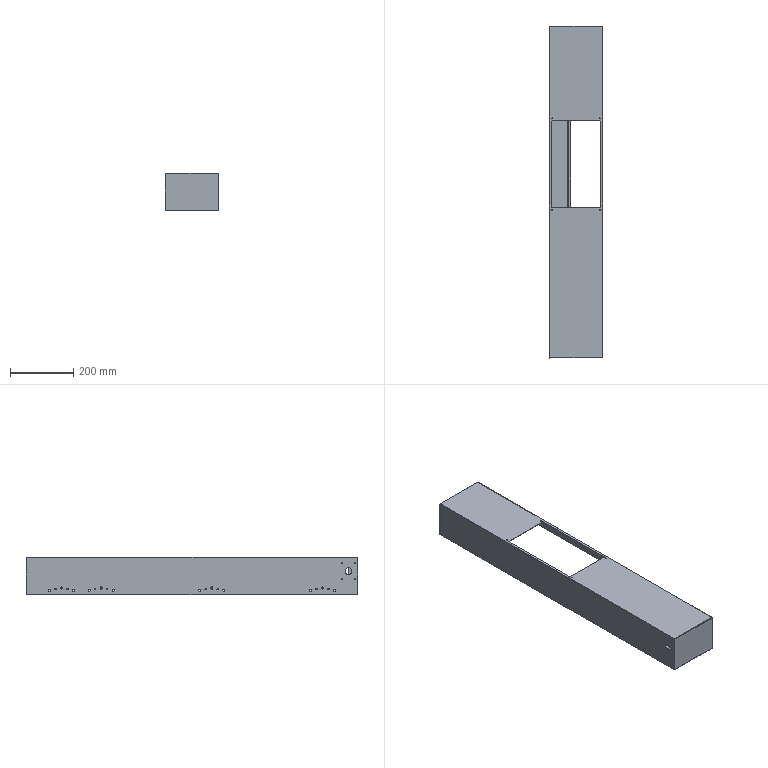Part | STEP file | HESS-408-70-15W-W-31-upper door left frame | 1 solid | 192 faces | box 170 x 1050 x 120 mm | volume 637779 mm3 | cylinder 92 | plane 84 | spline 16 | commonest cylinder face diameters 7 x24 3.3 x16 5 x16 0.2 x15 3.2 x15 6 x4